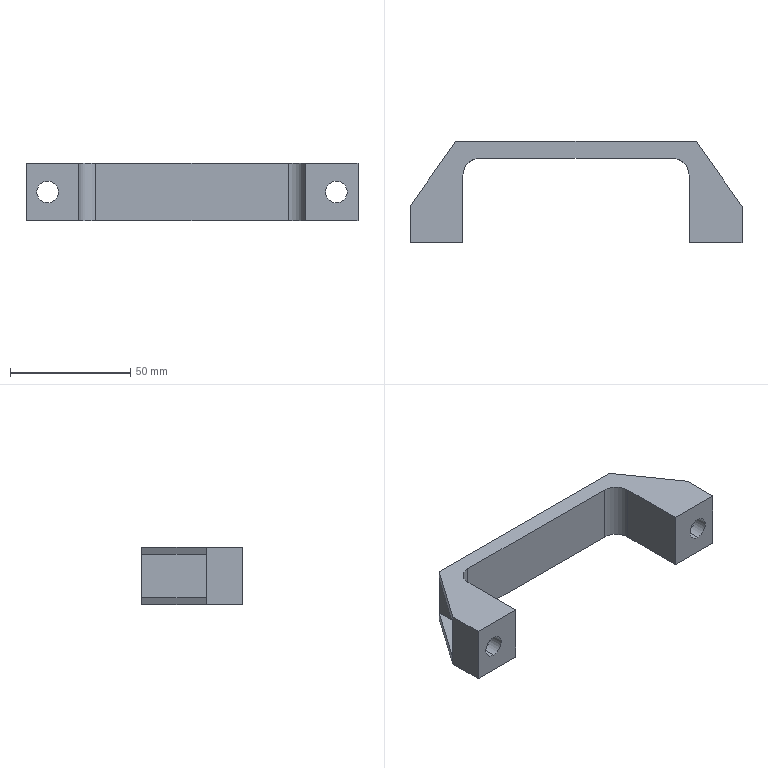Part | STEP file | Handle 180 | 1 solid | 34 faces | box 138 x 42 x 24 mm | volume 35568 mm3 | plane 24 | cylinder 10 | commonest cylinder face diameters 14 x6 9 x4